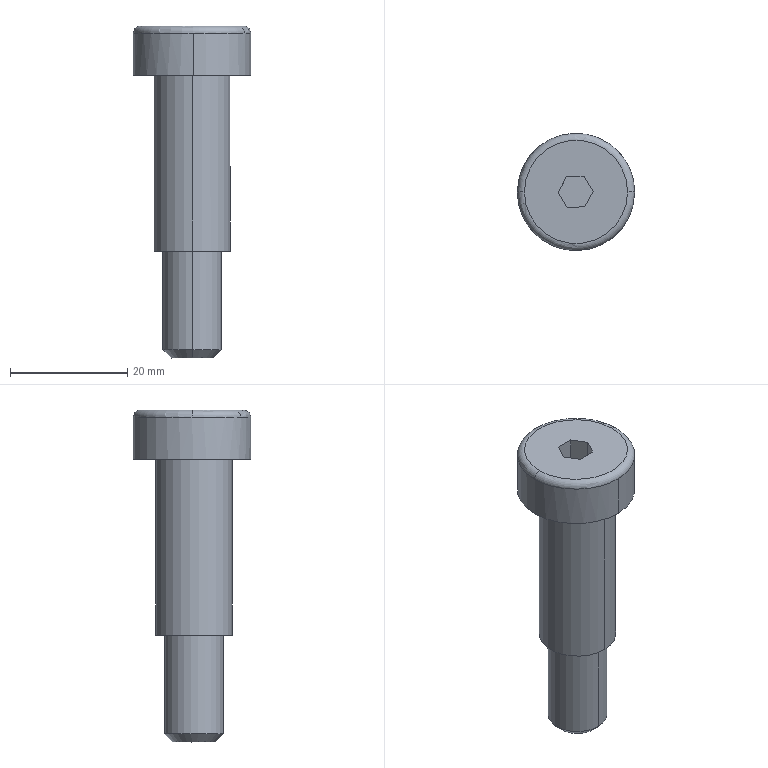Part | SolidWorks | features BaseBody 1 | 1 solid | 21 faces | box 20.001 x 20 x 56.624 mm | volume 7865 mm3 | plane 11 | cylinder 6 | torus 2 | cone 2 | commonest cylinder face diameters 10 x2 13 x2 20 x2
STEP:
#1=CARTESIAN_POINT('',(405.87,344.309,105.739));
#2=VERTEX_POINT('',#1);
#3=CARTESIAN_POINT('',(396.081,334.312,105.737));
#4=VERTEX_POINT('',#3);
#5=CARTESIAN_POINT('',(406.081,334.312,105.739));
#6=DIRECTION('',(-0.0001435,-0.000000521,1.));
#7=DIRECTION('',(0.02104,-0.9998,0.000002497));
#8=AXIS2_PLACEMENT_3D('',#5,#6,#7);
#9=CIRCLE('',#8,10.);
#10=EDGE_CURVE('',#2,#4,#9,.T.);
#11=ORIENTED_EDGE('',*,*,#10,.T.);
#12=CARTESIAN_POINT('',(397.281,334.312,106.937));
#13=VERTEX_POINT('',#12);
#14=CARTESIAN_POINT('',(397.281,334.312,105.737));
#15=DIRECTION('',(0.,1.,0.000000521));
#16=DIRECTION('',(0.,-0.000000521,1.));
#17=AXIS2_PLACEMENT_3D('',#14,#15,#16);
#18=CIRCLE('',#17,1.2);
#19=EDGE_CURVE('',#4,#13,#18,.T.);
#20=ORIENTED_EDGE('',*,*,#19,.T.);
#21=CARTESIAN_POINT('',(414.881,334.312,106.94));
#22=VERTEX_POINT('',#21);
#23=CARTESIAN_POINT('',(406.081,334.312,106.939));
#24=DIRECTION('',(-0.0001435,-0.000000521,1.));
#25=DIRECTION('',(-1.,0.,-0.0001435));
#26=AXIS2_PLACEMENT_3D('',#23,#24,#25);
#27=CIRCLE('',#26,8.8);
#28=EDGE_CURVE('',#22,#13,#27,.T.);
#29=ORIENTED_EDGE('',*,*,#28,.F.);
#30=CARTESIAN_POINT('',(416.081,334.312,105.74));
#31=VERTEX_POINT('',#30);
#32=CARTESIAN_POINT('',(414.881,334.312,105.74));
#33=DIRECTION('',(0.,-1.,-0.000000521));
#34=DIRECTION('',(0.,0.000000521,-1.));
#35=AXIS2_PLACEMENT_3D('',#32,#33,#34);
#36=CIRCLE('',#35,1.2);
#37=EDGE_CURVE('',#31,#22,#36,.T.);
#38=ORIENTED_EDGE('',*,*,#37,.F.);
#39=CARTESIAN_POINT('',(406.081,334.312,105.739));
#40=DIRECTION('',(-0.0001435,-0.000000521,1.));
#41=DIRECTION('',(0.02104,-0.9998,0.000002497));
#42=AXIS2_PLACEMENT_3D('',#39,#40,#41);
#43=CIRCLE('',#42,10.);
#44=EDGE_CURVE('',#31,#2,#43,.T.);
#45=ORIENTED_EDGE('',*,*,#44,.T.);
#46=EDGE_LOOP('',(#11,#20,#29,#38,#45));
#47=FACE_OUTER_BOUND('',#46,.T.);
#48=CARTESIAN_POINT('',(406.081,334.312,105.739));
#49=DIRECTION('',(-0.0001435,-0.000000521,1.));
#50=DIRECTION('',(1.,0.,0.0001435));
#51=AXIS2_PLACEMENT_3D('',#48,#49,#50);
#52=TOROIDAL_SURFACE('',#51,8.8,1.2);
#53=ADVANCED_FACE('',(#47),#52,.T.);
#54=CARTESIAN_POINT('',(406.292,324.314,98.539));
#55=VERTEX_POINT('',#54);
#56=CARTESIAN_POINT('',(405.871,344.309,98.539));
#57=VERTEX_POINT('',#56);
#58=CARTESIAN_POINT('',(406.082,334.312,98.539));
#59=DIRECTION('',(0.0001435,0.000000521,-1.));
#60=DIRECTION('',(-1.,0.,-0.0001435));
#61=AXIS2_PLACEMENT_3D('',#58,#59,#60);
#62=CIRCLE('',#61,10.);
#63=EDGE_CURVE('',#55,#57,#62,.T.);
#64=ORIENTED_EDGE('',*,*,#63,.F.);
#65=CARTESIAN_POINT('',(406.291,324.314,105.739));
#66=VERTEX_POINT('',#65);
#67=CARTESIAN_POINT('',(406.292,324.314,98.539));
#68=DIRECTION('',(-0.0001435,-0.000000521,1.));
#69=VECTOR('',#68,1000.);
#70=LINE('',#67,#69);
#71=EDGE_CURVE('',#55,#66,#70,.T.);
#72=ORIENTED_EDGE('',*,*,#71,.T.);
#73=CARTESIAN_POINT('',(406.081,334.312,105.739));
#74=DIRECTION('',(-0.0001435,-0.000000521,1.));
#75=DIRECTION('',(0.02104,-0.9998,0.000002497));
#76=AXIS2_PLACEMENT_3D('',#73,#74,#75);
#77=CIRCLE('',#76,10.);
#78=EDGE_CURVE('',#4,#66,#77,.T.);
#79=ORIENTED_EDGE('',*,*,#78,.F.);
#80=ORIENTED_EDGE('',*,*,#10,.F.);
#81=CARTESIAN_POINT('',(405.871,344.309,98.539));
#82=DIRECTION('',(-0.0001435,-0.000000521,1.));
#83=VECTOR('',#82,1000.);
#84=LINE('',#81,#83);
#85=EDGE_CURVE('',#57,#2,#84,.T.);
#86=ORIENTED_EDGE('',*,*,#85,.F.);
#87=EDGE_LOOP('',(#64,#72,#79,#80,#86));
#88=FACE_OUTER_BOUND('',#87,.T.);
#89=CARTESIAN_POINT('',(406.082,334.312,98.539));
#90=DIRECTION('',(-0.0001435,-0.000000521,1.));
#91=DIRECTION('',(-0.02104,0.9998,-0.000002497));
#92=AXIS2_PLACEMENT_3D('',#89,#90,#91);
#93=CYLINDRICAL_SURFACE('',#92,10.);
#94=ADVANCED_FACE('',(#88),#93,.T.);
#95=CARTESIAN_POINT('',(405.955,340.473,98.539));
#96=VERTEX_POINT('',#95);
#97=CARTESIAN_POINT('',(406.229,327.476,98.539));
#98=VERTEX_POINT('',#97);
#99=CARTESIAN_POINT('',(406.092,333.974,98.539));
#100=DIRECTION('',(-0.0001435,-0.000000521,1.));
#101=DIRECTION('',(0.02104,-0.9998,0.000002497));
#102=AXIS2_PLACEMENT_3D('',#99,#100,#101);
#103=CIRCLE('',#102,6.5);
#104=EDGE_CURVE('',#96,#98,#103,.T.);
#105=ORIENTED_EDGE('',*,*,#104,.F.);
#106=CARTESIAN_POINT('',(405.959,340.473,68.539));
#107=VERTEX_POINT('',#106);
#108=CARTESIAN_POINT('',(405.96,340.473,66.342));
#109=DIRECTION('',(0.0001435,0.000000521,-1.));
#110=VECTOR('',#109,1000.);
#111=LINE('',#108,#110);
#112=EDGE_CURVE('',#96,#107,#111,.T.);
#113=ORIENTED_EDGE('',*,*,#112,.T.);
#114=CARTESIAN_POINT('',(406.233,327.476,68.539));
#115=VERTEX_POINT('',#114);
#116=CARTESIAN_POINT('',(406.096,333.974,68.539));
#117=DIRECTION('',(0.0001435,0.000000521,-1.));
#118=DIRECTION('',(-1.,0.,-0.0001435));
#119=AXIS2_PLACEMENT_3D('',#116,#117,#118);
#120=CIRCLE('',#119,6.5);
#121=EDGE_CURVE('',#115,#107,#120,.T.);
#122=ORIENTED_EDGE('',*,*,#121,.F.);
#123=CARTESIAN_POINT('',(406.233,327.476,66.342));
#124=DIRECTION('',(0.0001435,0.000000521,-1.));
#125=VECTOR('',#124,1000.);
#126=LINE('',#123,#125);
#127=EDGE_CURVE('',#98,#115,#126,.T.);
#128=ORIENTED_EDGE('',*,*,#127,.F.);
#129=EDGE_LOOP('',(#105,#113,#122,#128));
#130=FACE_OUTER_BOUND('',#129,.T.);
#131=CARTESIAN_POINT('',(406.097,333.974,66.342));
#132=DIRECTION('',(0.0001435,0.000000521,-1.));
#133=DIRECTION('',(0.02104,-0.9998,0.000002497));
#134=AXIS2_PLACEMENT_3D('',#131,#132,#133);
#135=CYLINDRICAL_SURFACE('',#134,6.5);
#136=ADVANCED_FACE('',(#130),#135,.T.);
#137=CARTESIAN_POINT('',(405.994,338.973,68.539));
#138=VERTEX_POINT('',#137);
#139=CARTESIAN_POINT('',(406.204,328.975,68.539));
#140=VERTEX_POINT('',#139);
#141=CARTESIAN_POINT('',(406.099,333.974,68.539));
#142=DIRECTION('',(-0.0001435,-0.000000521,1.));
#143=DIRECTION('',(0.02104,-0.9998,0.000002497));
#144=AXIS2_PLACEMENT_3D('',#141,#142,#143);
#145=CIRCLE('',#144,5.);
#146=EDGE_CURVE('',#138,#140,#145,.T.);
#147=ORIENTED_EDGE('',*,*,#146,.F.);
#148=CARTESIAN_POINT('',(405.996,338.973,51.716));
#149=VERTEX_POINT('',#148);
#150=CARTESIAN_POINT('',(405.994,338.973,63.756));
#151=DIRECTION('',(0.0001435,0.000000521,-1.));
#152=VECTOR('',#151,1000.);
#153=LINE('',#150,#152);
#154=EDGE_CURVE('',#138,#149,#153,.T.);
#155=ORIENTED_EDGE('',*,*,#154,.T.);
#156=CARTESIAN_POINT('',(406.206,328.975,51.716));
#157=VERTEX_POINT('',#156);
#158=CARTESIAN_POINT('',(406.101,333.974,51.716));
#159=DIRECTION('',(0.0001435,0.000000521,-1.));
#160=DIRECTION('',(0.02104,-0.9998,0.000002497));
#161=AXIS2_PLACEMENT_3D('',#158,#159,#160);
#162=CIRCLE('',#161,5.);
#163=EDGE_CURVE('',#157,#149,#162,.T.);
#164=ORIENTED_EDGE('',*,*,#163,.F.);
#165=CARTESIAN_POINT('',(406.205,328.975,63.756));
#166=DIRECTION('',(0.0001435,0.000000521,-1.));
#167=VECTOR('',#166,1000.);
#168=LINE('',#165,#167);
#169=EDGE_CURVE('',#140,#157,#168,.T.);
#170=ORIENTED_EDGE('',*,*,#169,.F.);
#171=EDGE_LOOP('',(#147,#155,#164,#170));
#172=FACE_OUTER_BOUND('',#171,.T.);
#173=CARTESIAN_POINT('',(406.1,333.974,63.756));
#174=DIRECTION('',(0.0001435,0.000000521,-1.));
#175=DIRECTION('',(0.02104,-0.9998,0.000002497));
#176=AXIS2_PLACEMENT_3D('',#173,#174,#175);
#177=CYLINDRICAL_SURFACE('',#176,5.);
#178=ADVANCED_FACE('',(#172),#177,.T.);
#179=CARTESIAN_POINT('',(406.177,330.375,50.316));
#180=VERTEX_POINT('',#179);
#181=CARTESIAN_POINT('',(406.026,337.573,50.316));
#182=VERTEX_POINT('',#181);
#183=CARTESIAN_POINT('',(406.101,333.974,50.316));
#184=DIRECTION('',(0.0001435,0.000000521,-1.));
#185=DIRECTION('',(0.02104,-0.9998,0.000002497));
#186=AXIS2_PLACEMENT_3D('',#183,#184,#185);
#187=CIRCLE('',#186,3.6);
#188=EDGE_CURVE('',#180,#182,#187,.T.);
#189=ORIENTED_EDGE('',*,*,#188,.F.);
#190=CARTESIAN_POINT('',(406.192,329.675,51.016));
#191=DIRECTION('',(0.01477,-0.707,0.7071));
#192=VECTOR('',#191,1000.);
#193=LINE('',#190,#192);
#194=EDGE_CURVE('',#180,#157,#193,.T.);
#195=ORIENTED_EDGE('',*,*,#194,.T.);
#196=ORIENTED_EDGE('',*,*,#163,.T.);
#197=CARTESIAN_POINT('',(406.011,338.273,51.016));
#198=DIRECTION('',(-0.01498,0.7069,0.7071));
#199=VECTOR('',#198,1000.);
#200=LINE('',#197,#199);
#201=EDGE_CURVE('',#182,#149,#200,.T.);
#202=ORIENTED_EDGE('',*,*,#201,.F.);
#203=EDGE_LOOP('',(#189,#195,#196,#202));
#204=FACE_OUTER_BOUND('',#203,.T.);
#205=CARTESIAN_POINT('',(406.101,333.974,51.016));
#206=DIRECTION('',(-0.0001435,-0.000000521,1.));
#207=DIRECTION('',(-0.02104,0.9998,-0.000002497));
#208=AXIS2_PLACEMENT_3D('',#205,#206,#207);
#209=CONICAL_SURFACE('',#208,4.3,0.7854);
#210=ADVANCED_FACE('',(#204),#209,.T.);
#211=CARTESIAN_POINT('',(406.101,333.974,50.316));
#212=DIRECTION('',(0.0001435,0.000000521,-1.));
#213=DIRECTION('',(0.02104,-0.9998,0.000002497));
#214=AXIS2_PLACEMENT_3D('',#211,#212,#213);
#215=CIRCLE('',#214,3.6);
#216=EDGE_CURVE('',#182,#180,#215,.T.);
#217=ORIENTED_EDGE('',*,*,#216,.T.);
#218=ORIENTED_EDGE('',*,*,#188,.T.);
#219=EDGE_LOOP('',(#217,#218));
#220=FACE_OUTER_BOUND('',#219,.T.);
#221=CARTESIAN_POINT('',(406.101,333.974,50.316));
#222=DIRECTION('',(0.0001435,0.000000521,-1.));
#223=DIRECTION('',(0.,-1.,-0.000000521));
#224=AXIS2_PLACEMENT_3D('',#221,#222,#223);
#225=PLANE('',#224);
#226=ADVANCED_FACE('',(#220),#225,.T.);
#227=ORIENTED_EDGE('',*,*,#194,.F.);
#228=ORIENTED_EDGE('',*,*,#216,.F.);
#229=ORIENTED_EDGE('',*,*,#201,.T.);
#230=CARTESIAN_POINT('',(406.101,333.974,51.716));
#231=DIRECTION('',(0.0001435,0.000000521,-1.));
#232=DIRECTION('',(0.02104,-0.9998,0.000002497));
#233=AXIS2_PLACEMENT_3D('',#230,#231,#232);
#234=CIRCLE('',#233,5.);
#235=EDGE_CURVE('',#149,#157,#234,.T.);
#236=ORIENTED_EDGE('',*,*,#235,.T.);
#237=EDGE_LOOP('',(#227,#228,#229,#236));
#238=FACE_OUTER_BOUND('',#237,.T.);
#239=CARTESIAN_POINT('',(406.101,333.974,51.016));
#240=DIRECTION('',(-0.0001435,-0.000000521,1.));
#241=DIRECTION('',(-0.02104,0.9998,-0.000002497));
#242=AXIS2_PLACEMENT_3D('',#239,#240,#241);
#243=CONICAL_SURFACE('',#242,4.3,0.7854);
#244=ADVANCED_FACE('',(#238),#243,.T.);
#245=ORIENTED_EDGE('',*,*,#154,.F.);
#246=CARTESIAN_POINT('',(406.099,333.974,68.539));
#247=DIRECTION('',(-0.0001435,-0.000000521,1.));
#248=DIRECTION('',(0.02104,-0.9998,0.000002497));
#249=AXIS2_PLACEMENT_3D('',#246,#247,#248);
#250=CIRCLE('',#249,5.);
#251=EDGE_CURVE('',#140,#138,#250,.T.);
#252=ORIENTED_EDGE('',*,*,#251,.F.);
#253=ORIENTED_EDGE('',*,*,#169,.T.);
#254=ORIENTED_EDGE('',*,*,#235,.F.);
#255=EDGE_LOOP('',(#245,#252,#253,#254));
#256=FACE_OUTER_BOUND('',#255,.T.);
#257=CARTESIAN_POINT('',(406.1,333.974,63.756));
#258=DIRECTION('',(0.0001435,0.000000521,-1.));
#259=DIRECTION('',(0.02104,-0.9998,0.000002497));
#260=AXIS2_PLACEMENT_3D('',#257,#258,#259);
#261=CYLINDRICAL_SURFACE('',#260,5.);
#262=ADVANCED_FACE('',(#256),#261,.T.);
#263=ORIENTED_EDGE('',*,*,#251,.T.);
#264=ORIENTED_EDGE('',*,*,#146,.T.);
#265=EDGE_LOOP('',(#263,#264));
#266=FACE_BOUND('',#265,.T.);
#267=ORIENTED_EDGE('',*,*,#121,.T.);
#268=CARTESIAN_POINT('',(406.096,333.974,68.539));
#269=DIRECTION('',(0.0001435,0.000000521,-1.));
#270=DIRECTION('',(-1.,0.,-0.0001435));
#271=AXIS2_PLACEMENT_3D('',#268,#269,#270);
#272=CIRCLE('',#271,6.5);
#273=EDGE_CURVE('',#107,#115,#272,.T.);
#274=ORIENTED_EDGE('',*,*,#273,.T.);
#275=EDGE_LOOP('',(#267,#274));
#276=FACE_OUTER_BOUND('',#275,.T.);
#277=CARTESIAN_POINT('',(406.086,334.312,68.539));
#278=DIRECTION('',(0.0001435,0.000000521,-1.));
#279=DIRECTION('',(0.,-1.,-0.000000521));
#280=AXIS2_PLACEMENT_3D('',#277,#278,#279);
#281=PLANE('',#280);
#282=ADVANCED_FACE('',(#266,#276),#281,.T.);
#283=ORIENTED_EDGE('',*,*,#112,.F.);
#284=CARTESIAN_POINT('',(406.092,333.974,98.539));
#285=DIRECTION('',(-0.0001435,-0.000000521,1.));
#286=DIRECTION('',(0.02104,-0.9998,0.000002497));
#287=AXIS2_PLACEMENT_3D('',#284,#285,#286);
#288=CIRCLE('',#287,6.5);
#289=EDGE_CURVE('',#98,#96,#288,.T.);
#290=ORIENTED_EDGE('',*,*,#289,.F.);
#291=ORIENTED_EDGE('',*,*,#127,.T.);
#292=ORIENTED_EDGE('',*,*,#273,.F.);
#293=EDGE_LOOP('',(#283,#290,#291,#292));
#294=FACE_OUTER_BOUND('',#293,.T.);
#295=CARTESIAN_POINT('',(406.097,333.974,66.342));
#296=DIRECTION('',(0.0001435,0.000000521,-1.));
#297=DIRECTION('',(0.02104,-0.9998,0.000002497));
#298=AXIS2_PLACEMENT_3D('',#295,#296,#297);
#299=CYLINDRICAL_SURFACE('',#298,6.5);
#300=ADVANCED_FACE('',(#294),#299,.T.);
#301=ORIENTED_EDGE('',*,*,#289,.T.);
#302=ORIENTED_EDGE('',*,*,#104,.T.);
#303=EDGE_LOOP('',(#301,#302));
#304=FACE_BOUND('',#303,.T.);
#305=CARTESIAN_POINT('',(406.082,334.312,98.539));
#306=DIRECTION('',(0.0001435,0.000000521,-1.));
#307=DIRECTION('',(-1.,0.,-0.0001435));
#308=AXIS2_PLACEMENT_3D('',#305,#306,#307);
#309=CIRCLE('',#308,10.);
#310=EDGE_CURVE('',#57,#55,#309,.T.);
#311=ORIENTED_EDGE('',*,*,#310,.T.);
#312=ORIENTED_EDGE('',*,*,#63,.T.);
#313=EDGE_LOOP('',(#311,#312));
#314=FACE_OUTER_BOUND('',#313,.T.);
#315=CARTESIAN_POINT('',(406.082,334.312,98.539));
#316=DIRECTION('',(0.0001435,0.000000521,-1.));
#317=DIRECTION('',(0.,-1.,-0.000000521));
#318=AXIS2_PLACEMENT_3D('',#315,#316,#317);
#319=PLANE('',#318);
#320=ADVANCED_FACE('',(#304,#314),#319,.T.);
#321=ORIENTED_EDGE('',*,*,#71,.F.);
#322=ORIENTED_EDGE('',*,*,#310,.F.);
#323=ORIENTED_EDGE('',*,*,#85,.T.);
#324=ORIENTED_EDGE('',*,*,#44,.F.);
#325=CARTESIAN_POINT('',(406.081,334.312,105.739));
#326=DIRECTION('',(-0.0001435,-0.000000521,1.));
#327=DIRECTION('',(0.02104,-0.9998,0.000002497));
#328=AXIS2_PLACEMENT_3D('',#325,#326,#327);
#329=CIRCLE('',#328,10.);
#330=EDGE_CURVE('',#66,#31,#329,.T.);
#331=ORIENTED_EDGE('',*,*,#330,.F.);
#332=EDGE_LOOP('',(#321,#322,#323,#324,#331));
#333=FACE_OUTER_BOUND('',#332,.T.);
#334=CARTESIAN_POINT('',(406.082,334.312,98.539));
#335=DIRECTION('',(-0.0001435,-0.000000521,1.));
#336=DIRECTION('',(-0.02104,0.9998,-0.000002497));
#337=AXIS2_PLACEMENT_3D('',#334,#335,#336);
#338=CYLINDRICAL_SURFACE('',#337,10.);
#339=ADVANCED_FACE('',(#333),#338,.T.);
#340=ORIENTED_EDGE('',*,*,#19,.F.);
#341=ORIENTED_EDGE('',*,*,#78,.T.);
#342=ORIENTED_EDGE('',*,*,#330,.T.);
#343=ORIENTED_EDGE('',*,*,#37,.T.);
#344=CARTESIAN_POINT('',(406.081,334.312,106.939));
#345=DIRECTION('',(-0.0001435,-0.000000521,1.));
#346=DIRECTION('',(-1.,0.,-0.0001435));
#347=AXIS2_PLACEMENT_3D('',#344,#345,#346);
#348=CIRCLE('',#347,8.8);
#349=EDGE_CURVE('',#13,#22,#348,.T.);
#350=ORIENTED_EDGE('',*,*,#349,.F.);
#351=EDGE_LOOP('',(#340,#341,#342,#343,#350));
#352=FACE_OUTER_BOUND('',#351,.T.);
#353=CARTESIAN_POINT('',(406.081,334.312,105.739));
#354=DIRECTION('',(-0.0001435,-0.000000521,1.));
#355=DIRECTION('',(1.,0.,0.0001435));
#356=AXIS2_PLACEMENT_3D('',#353,#354,#355);
#357=TOROIDAL_SURFACE('',#356,8.8,1.2);
#358=ADVANCED_FACE('',(#352),#357,.T.);
#359=CARTESIAN_POINT('',(404.579,331.701,100.938));
#360=VERTEX_POINT('',#359);
#361=CARTESIAN_POINT('',(407.579,331.764,100.939));
#362=VERTEX_POINT('',#361);
#363=CARTESIAN_POINT('',(404.579,331.701,100.938));
#364=DIRECTION('',(0.9998,0.02104,0.0001435));
#365=VECTOR('',#364,1000.);
#366=LINE('',#363,#365);
#367=EDGE_CURVE('',#360,#362,#366,.T.);
#368=ORIENTED_EDGE('',*,*,#367,.T.);
#369=CARTESIAN_POINT('',(409.024,334.393,100.939));
#370=VERTEX_POINT('',#369);
#371=CARTESIAN_POINT('',(407.579,331.764,100.939));
#372=DIRECTION('',(0.4817,0.8764,0.00006956));
#373=VECTOR('',#372,1000.);
#374=LINE('',#371,#373);
#375=EDGE_CURVE('',#362,#370,#374,.T.);
#376=ORIENTED_EDGE('',*,*,#375,.T.);
#377=CARTESIAN_POINT('',(407.469,336.959,100.939));
#378=VERTEX_POINT('',#377);
#379=CARTESIAN_POINT('',(409.024,334.393,100.939));
#380=DIRECTION('',(-0.5181,0.8553,-0.00007389));
#381=VECTOR('',#380,1000.);
#382=LINE('',#379,#381);
#383=EDGE_CURVE('',#370,#378,#382,.T.);
#384=ORIENTED_EDGE('',*,*,#383,.T.);
#385=CARTESIAN_POINT('',(404.47,336.896,100.938));
#386=VERTEX_POINT('',#385);
#387=CARTESIAN_POINT('',(407.469,336.959,100.939));
#388=DIRECTION('',(-0.9998,-0.02104,-0.0001435));
#389=VECTOR('',#388,1000.);
#390=LINE('',#387,#389);
#391=EDGE_CURVE('',#378,#386,#390,.T.);
#392=ORIENTED_EDGE('',*,*,#391,.T.);
#393=CARTESIAN_POINT('',(403.025,334.267,100.938));
#394=VERTEX_POINT('',#393);
#395=CARTESIAN_POINT('',(404.47,336.896,100.938));
#396=DIRECTION('',(-0.4817,-0.8764,-0.00006956));
#397=VECTOR('',#396,1000.);
#398=LINE('',#395,#397);
#399=EDGE_CURVE('',#386,#394,#398,.T.);
#400=ORIENTED_EDGE('',*,*,#399,.T.);
#401=CARTESIAN_POINT('',(403.025,334.267,100.938));
#402=DIRECTION('',(0.5181,-0.8553,0.00007389));
#403=VECTOR('',#402,1000.);
#404=LINE('',#401,#403);
#405=EDGE_CURVE('',#394,#360,#404,.T.);
#406=ORIENTED_EDGE('',*,*,#405,.T.);
#407=EDGE_LOOP('',(#368,#376,#384,#392,#400,#406));
#408=FACE_OUTER_BOUND('',#407,.T.);
#409=CARTESIAN_POINT('',(405.469,363.405,100.939));
#410=DIRECTION('',(-0.0001435,-0.000000521,1.));
#411=DIRECTION('',(-0.003633,1.,0.));
#412=AXIS2_PLACEMENT_3D('',#409,#410,#411);
#413=PLANE('',#412);
#414=ADVANCED_FACE('',(#408),#413,.T.);
#415=CARTESIAN_POINT('',(407.578,331.764,106.939));
#416=VERTEX_POINT('',#415);
#417=CARTESIAN_POINT('',(407.578,331.764,106.939));
#418=DIRECTION('',(0.0001435,0.000000521,-1.));
#419=VECTOR('',#418,1000.);
#420=LINE('',#417,#419);
#421=EDGE_CURVE('',#416,#362,#420,.T.);
#422=ORIENTED_EDGE('',*,*,#421,.T.);
#423=ORIENTED_EDGE('',*,*,#367,.F.);
#424=CARTESIAN_POINT('',(404.578,331.701,106.938));
#425=VERTEX_POINT('',#424);
#426=CARTESIAN_POINT('',(404.578,331.701,106.938));
#427=DIRECTION('',(0.0001435,0.000000521,-1.));
#428=VECTOR('',#427,1000.);
#429=LINE('',#426,#428);
#430=EDGE_CURVE('',#425,#360,#429,.T.);
#431=ORIENTED_EDGE('',*,*,#430,.F.);
#432=CARTESIAN_POINT('',(407.578,331.764,106.939));
#433=DIRECTION('',(-0.9998,-0.02104,-0.0001435));
#434=VECTOR('',#433,1000.);
#435=LINE('',#432,#434);
#436=EDGE_CURVE('',#416,#425,#435,.T.);
#437=ORIENTED_EDGE('',*,*,#436,.F.);
#438=EDGE_LOOP('',(#422,#423,#431,#437));
#439=FACE_OUTER_BOUND('',#438,.T.);
#440=CARTESIAN_POINT('',(407.579,331.764,100.939));
#441=DIRECTION('',(0.02104,-0.9998,0.000002497));
#442=DIRECTION('',(0.,-0.000002498,-1.));
#443=AXIS2_PLACEMENT_3D('',#440,#441,#442);
#444=PLANE('',#443);
#445=ADVANCED_FACE('',(#439),#444,.F.);
#446=CARTESIAN_POINT('',(409.023,334.393,106.939));
#447=VERTEX_POINT('',#446);
#448=CARTESIAN_POINT('',(409.023,334.393,106.939));
#449=DIRECTION('',(0.0001435,0.000000521,-1.));
#450=VECTOR('',#449,1000.);
#451=LINE('',#448,#450);
#452=EDGE_CURVE('',#447,#370,#451,.T.);
#453=ORIENTED_EDGE('',*,*,#452,.T.);
#454=ORIENTED_EDGE('',*,*,#375,.F.);
#455=ORIENTED_EDGE('',*,*,#421,.F.);
#456=CARTESIAN_POINT('',(409.023,334.393,106.939));
#457=DIRECTION('',(-0.4817,-0.8764,-0.00006956));
#458=VECTOR('',#457,1000.);
#459=LINE('',#456,#458);
#460=EDGE_CURVE('',#447,#416,#459,.T.);
#461=ORIENTED_EDGE('',*,*,#460,.F.);
#462=EDGE_LOOP('',(#453,#454,#455,#461));
#463=FACE_OUTER_BOUND('',#462,.T.);
#464=CARTESIAN_POINT('',(409.024,334.393,100.939));
#465=DIRECTION('',(0.8764,-0.4817,0.0001255));
#466=DIRECTION('',(0.,-0.0002605,-1.));
#467=AXIS2_PLACEMENT_3D('',#464,#465,#466);
#468=PLANE('',#467);
#469=ADVANCED_FACE('',(#463),#468,.F.);
#470=CARTESIAN_POINT('',(407.468,336.959,106.939));
#471=VERTEX_POINT('',#470);
#472=CARTESIAN_POINT('',(407.468,336.959,106.939));
#473=DIRECTION('',(0.0001435,0.000000521,-1.));
#474=VECTOR('',#473,1000.);
#475=LINE('',#472,#474);
#476=EDGE_CURVE('',#471,#378,#475,.T.);
#477=ORIENTED_EDGE('',*,*,#476,.T.);
#478=ORIENTED_EDGE('',*,*,#383,.F.);
#479=ORIENTED_EDGE('',*,*,#452,.F.);
#480=CARTESIAN_POINT('',(407.468,336.959,106.939));
#481=DIRECTION('',(0.5181,-0.8553,0.00007389));
#482=VECTOR('',#481,1000.);
#483=LINE('',#480,#482);
#484=EDGE_CURVE('',#471,#447,#483,.T.);
#485=ORIENTED_EDGE('',*,*,#484,.F.);
#486=EDGE_LOOP('',(#477,#478,#479,#485));
#487=FACE_OUTER_BOUND('',#486,.T.);
#488=CARTESIAN_POINT('',(407.469,336.959,100.939));
#489=DIRECTION('',(0.8553,0.5181,0.000123));
#490=DIRECTION('',(0.,0.0002374,-1.));
#491=AXIS2_PLACEMENT_3D('',#488,#489,#490);
#492=PLANE('',#491);
#493=ADVANCED_FACE('',(#487),#492,.F.);
#494=CARTESIAN_POINT('',(404.469,336.896,106.938));
#495=VERTEX_POINT('',#494);
#496=CARTESIAN_POINT('',(404.469,336.896,106.938));
#497=DIRECTION('',(0.0001435,0.000000521,-1.));
#498=VECTOR('',#497,1000.);
#499=LINE('',#496,#498);
#500=EDGE_CURVE('',#495,#386,#499,.T.);
#501=ORIENTED_EDGE('',*,*,#500,.T.);
#502=ORIENTED_EDGE('',*,*,#391,.F.);
#503=ORIENTED_EDGE('',*,*,#476,.F.);
#504=CARTESIAN_POINT('',(404.469,336.896,106.938));
#505=DIRECTION('',(0.9998,0.02104,0.0001435));
#506=VECTOR('',#505,1000.);
#507=LINE('',#504,#506);
#508=EDGE_CURVE('',#495,#471,#507,.T.);
#509=ORIENTED_EDGE('',*,*,#508,.F.);
#510=EDGE_LOOP('',(#501,#502,#503,#509));
#511=FACE_OUTER_BOUND('',#510,.T.);
#512=CARTESIAN_POINT('',(404.47,336.896,100.938));
#513=DIRECTION('',(-0.02104,0.9998,-0.000002497));
#514=DIRECTION('',(-0.0001187,0.,1.));
#515=AXIS2_PLACEMENT_3D('',#512,#513,#514);
#516=PLANE('',#515);
#517=ADVANCED_FACE('',(#511),#516,.F.);
#518=CARTESIAN_POINT('',(403.024,334.267,106.938));
#519=VERTEX_POINT('',#518);
#520=CARTESIAN_POINT('',(403.024,334.267,106.938));
#521=DIRECTION('',(0.0001435,0.000000521,-1.));
#522=VECTOR('',#521,1000.);
#523=LINE('',#520,#522);
#524=EDGE_CURVE('',#519,#394,#523,.T.);
#525=ORIENTED_EDGE('',*,*,#524,.T.);
#526=ORIENTED_EDGE('',*,*,#399,.F.);
#527=ORIENTED_EDGE('',*,*,#500,.F.);
#528=CARTESIAN_POINT('',(403.024,334.267,106.938));
#529=DIRECTION('',(0.4817,0.8764,0.00006956));
#530=VECTOR('',#529,1000.);
#531=LINE('',#528,#530);
#532=EDGE_CURVE('',#519,#495,#531,.T.);
#533=ORIENTED_EDGE('',*,*,#532,.F.);
#534=EDGE_LOOP('',(#525,#526,#527,#533));
#535=FACE_OUTER_BOUND('',#534,.T.);
#536=CARTESIAN_POINT('',(403.025,334.267,100.938));
#537=DIRECTION('',(-0.8764,0.4817,-0.0001255));
#538=DIRECTION('',(-0.0001432,0.,1.));
#539=AXIS2_PLACEMENT_3D('',#536,#537,#538);
#540=PLANE('',#539);
#541=ADVANCED_FACE('',(#535),#540,.F.);
#542=ORIENTED_EDGE('',*,*,#430,.T.);
#543=ORIENTED_EDGE('',*,*,#405,.F.);
#544=ORIENTED_EDGE('',*,*,#524,.F.);
#545=CARTESIAN_POINT('',(404.578,331.701,106.938));
#546=DIRECTION('',(-0.5181,0.8553,-0.00007389));
#547=VECTOR('',#546,1000.);
#548=LINE('',#545,#547);
#549=EDGE_CURVE('',#425,#519,#548,.T.);
#550=ORIENTED_EDGE('',*,*,#549,.F.);
#551=EDGE_LOOP('',(#542,#543,#544,#550));
#552=FACE_OUTER_BOUND('',#551,.T.);
#553=CARTESIAN_POINT('',(404.579,331.701,100.938));
#554=DIRECTION('',(-0.8553,-0.5181,-0.000123));
#555=DIRECTION('',(-0.5181,0.8553,0.));
#556=AXIS2_PLACEMENT_3D('',#553,#554,#555);
#557=PLANE('',#556);
#558=ADVANCED_FACE('',(#552),#557,.F.);
#559=ORIENTED_EDGE('',*,*,#532,.T.);
#560=ORIENTED_EDGE('',*,*,#508,.T.);
#561=ORIENTED_EDGE('',*,*,#484,.T.);
#562=ORIENTED_EDGE('',*,*,#460,.T.);
#563=ORIENTED_EDGE('',*,*,#436,.T.);
#564=ORIENTED_EDGE('',*,*,#549,.T.);
#565=EDGE_LOOP('',(#559,#560,#561,#562,#563,#564));
#566=FACE_BOUND('',#565,.T.);
#567=ORIENTED_EDGE('',*,*,#28,.T.);
#568=ORIENTED_EDGE('',*,*,#349,.T.);
#569=EDGE_LOOP('',(#567,#568));
#570=FACE_OUTER_BOUND('',#569,.T.);
#571=CARTESIAN_POINT('',(406.081,334.312,106.939));
#572=DIRECTION('',(-0.0001435,-0.000000521,1.));
#573=DIRECTION('',(-0.003633,1.,0.));
#574=AXIS2_PLACEMENT_3D('',#571,#572,#573);
#575=PLANE('',#574);
#576=ADVANCED_FACE('',(#566,#570),#575,.T.);
#577=CLOSED_SHELL('',(#53,#94,#136,#178,#210,#226,#244,#262,#282,#300,#320,#339,#358,#414,#445,#469,#493,#517,#541,#558,#576));
#578=MANIFOLD_SOLID_BREP('',#577);
#579=CARTESIAN_POINT('',(0.,0.,0.));
#580=DIRECTION('',(0.,0.,1.));
#581=DIRECTION('',(1.,0.,0.));
#582=AXIS2_PLACEMENT_3D('',#579,#580,#581);
#583=(LENGTH_UNIT()NAMED_UNIT(*)SI_UNIT(.MILLI.,.METRE.));
#584=UNCERTAINTY_MEASURE_WITH_UNIT(LENGTH_MEASURE(0.00001),#583,'','');
#585=(NAMED_UNIT(*)PLANE_ANGLE_UNIT()SI_UNIT($,.RADIAN.));
#586=(NAMED_UNIT(*)SI_UNIT($,.STERADIAN.)SOLID_ANGLE_UNIT());
#587=(GEOMETRIC_REPRESENTATION_CONTEXT(3)GLOBAL_UNCERTAINTY_ASSIGNED_CONTEXT((#584))GLOBAL_UNIT_ASSIGNED_CONTEXT((#583,#585,#586))REPRESENTATION_CONTEXT('',''));
#588=ADVANCED_BREP_SHAPE_REPRESENTATION('',(#578,#582),#587);